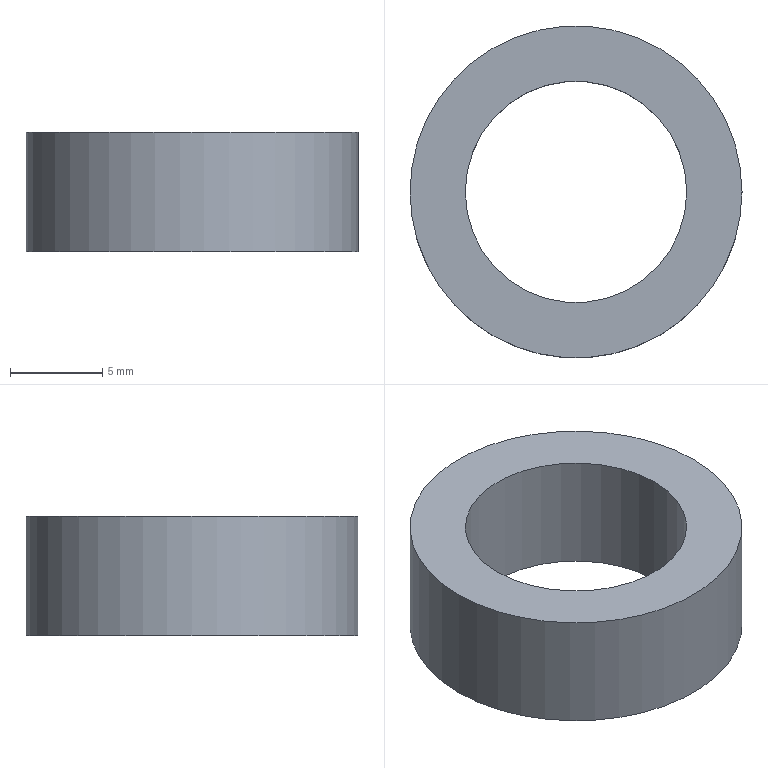Part | NX | features solid 2 | 1 solid | 4 faces | box 18 x 18 x 6.5 mm | volume 918.916 mm3 | plane 2 | cylinder 2 | commonest cylinder face diameters 12 x1 18 x1
STEP:
#1=CARTESIAN_POINT('',(679.,10.,-58.5));
#2=VERTEX_POINT('',#1);
#3=CARTESIAN_POINT('',(670.,10.,-58.5));
#4=DIRECTION('',(0.,0.,1.));
#5=DIRECTION('',(1.,0.,0.));
#6=AXIS2_PLACEMENT_3D('',#3,#4,#5);
#7=CIRCLE('',#6,9.);
#8=EDGE_CURVE('',#2,#2,#7,.T.);
#9=ORIENTED_EDGE('',*,*,#8,.T.);
#10=EDGE_LOOP('',(#9));
#11=FACE_BOUND('',#10,.T.);
#12=CARTESIAN_POINT('',(676.,10.,-58.5));
#13=VERTEX_POINT('',#12);
#14=CARTESIAN_POINT('',(670.,10.,-58.5));
#15=DIRECTION('',(0.,0.,1.));
#16=DIRECTION('',(1.,0.,0.));
#17=AXIS2_PLACEMENT_3D('',#14,#15,#16);
#18=CIRCLE('',#17,6.);
#19=EDGE_CURVE('',#13,#13,#18,.F.);
#20=ORIENTED_EDGE('',*,*,#19,.T.);
#21=EDGE_LOOP('',(#20));
#22=FACE_BOUND('',#21,.T.);
#23=CARTESIAN_POINT('',(670.,10.,-58.5));
#24=DIRECTION('',(0.,0.,1.));
#25=DIRECTION('',(1.,0.,0.));
#26=AXIS2_PLACEMENT_3D('',#23,#24,#25);
#27=PLANE('',#26);
#28=ADVANCED_FACE('',(#11,#22),#27,.T.);
#29=CARTESIAN_POINT('',(679.,10.,-65.));
#30=VERTEX_POINT('',#29);
#31=CARTESIAN_POINT('',(670.,10.,-65.));
#32=DIRECTION('',(0.,0.,1.));
#33=DIRECTION('',(1.,0.,0.));
#34=AXIS2_PLACEMENT_3D('',#31,#32,#33);
#35=CIRCLE('',#34,9.);
#36=EDGE_CURVE('',#30,#30,#35,.T.);
#37=ORIENTED_EDGE('',*,*,#36,.F.);
#38=EDGE_LOOP('',(#37));
#39=FACE_BOUND('',#38,.T.);
#40=CARTESIAN_POINT('',(676.,10.,-65.));
#41=VERTEX_POINT('',#40);
#42=CARTESIAN_POINT('',(670.,10.,-65.));
#43=DIRECTION('',(0.,0.,1.));
#44=DIRECTION('',(1.,0.,0.));
#45=AXIS2_PLACEMENT_3D('',#42,#43,#44);
#46=CIRCLE('',#45,6.);
#47=EDGE_CURVE('',#41,#41,#46,.T.);
#48=ORIENTED_EDGE('',*,*,#47,.T.);
#49=EDGE_LOOP('',(#48));
#50=FACE_BOUND('',#49,.T.);
#51=CARTESIAN_POINT('',(670.,10.,-65.));
#52=DIRECTION('',(0.,0.,1.));
#53=DIRECTION('',(1.,0.,0.));
#54=AXIS2_PLACEMENT_3D('',#51,#52,#53);
#55=PLANE('',#54);
#56=ADVANCED_FACE('',(#39,#50),#55,.F.);
#57=ORIENTED_EDGE('',*,*,#8,.F.);
#58=EDGE_LOOP('',(#57));
#59=FACE_BOUND('',#58,.T.);
#60=ORIENTED_EDGE('',*,*,#36,.T.);
#61=EDGE_LOOP('',(#60));
#62=FACE_BOUND('',#61,.T.);
#63=CARTESIAN_POINT('',(670.,10.,-58.5));
#64=DIRECTION('',(0.,0.,-1.));
#65=DIRECTION('',(-1.,0.,0.));
#66=AXIS2_PLACEMENT_3D('',#63,#64,#65);
#67=CYLINDRICAL_SURFACE('',#66,9.);
#68=ADVANCED_FACE('',(#59,#62),#67,.T.);
#69=ORIENTED_EDGE('',*,*,#19,.F.);
#70=EDGE_LOOP('',(#69));
#71=FACE_BOUND('',#70,.T.);
#72=ORIENTED_EDGE('',*,*,#47,.F.);
#73=EDGE_LOOP('',(#72));
#74=FACE_BOUND('',#73,.T.);
#75=CARTESIAN_POINT('',(670.,10.,-15.));
#76=DIRECTION('',(0.,0.,-1.));
#77=DIRECTION('',(-1.,0.,0.));
#78=AXIS2_PLACEMENT_3D('',#75,#76,#77);
#79=CYLINDRICAL_SURFACE('',#78,6.);
#80=ADVANCED_FACE('',(#71,#74),#79,.F.);
#81=CLOSED_SHELL('',(#28,#56,#68,#80));
#82=MANIFOLD_SOLID_BREP('',#81);
#83=(LENGTH_UNIT()NAMED_UNIT(*)SI_UNIT(.MILLI.,.METRE.));
#84=UNCERTAINTY_MEASURE_WITH_UNIT(LENGTH_MEASURE(0.00001),#83,'','');
#85=(NAMED_UNIT(*)PLANE_ANGLE_UNIT()SI_UNIT($,.RADIAN.));
#86=(NAMED_UNIT(*)SI_UNIT($,.STERADIAN.)SOLID_ANGLE_UNIT());
#87=(GEOMETRIC_REPRESENTATION_CONTEXT(3)GLOBAL_UNCERTAINTY_ASSIGNED_CONTEXT((#84))GLOBAL_UNIT_ASSIGNED_CONTEXT((#83,#85,#86))REPRESENTATION_CONTEXT('',''));
#88=ADVANCED_BREP_SHAPE_REPRESENTATION('',(#82),#87);